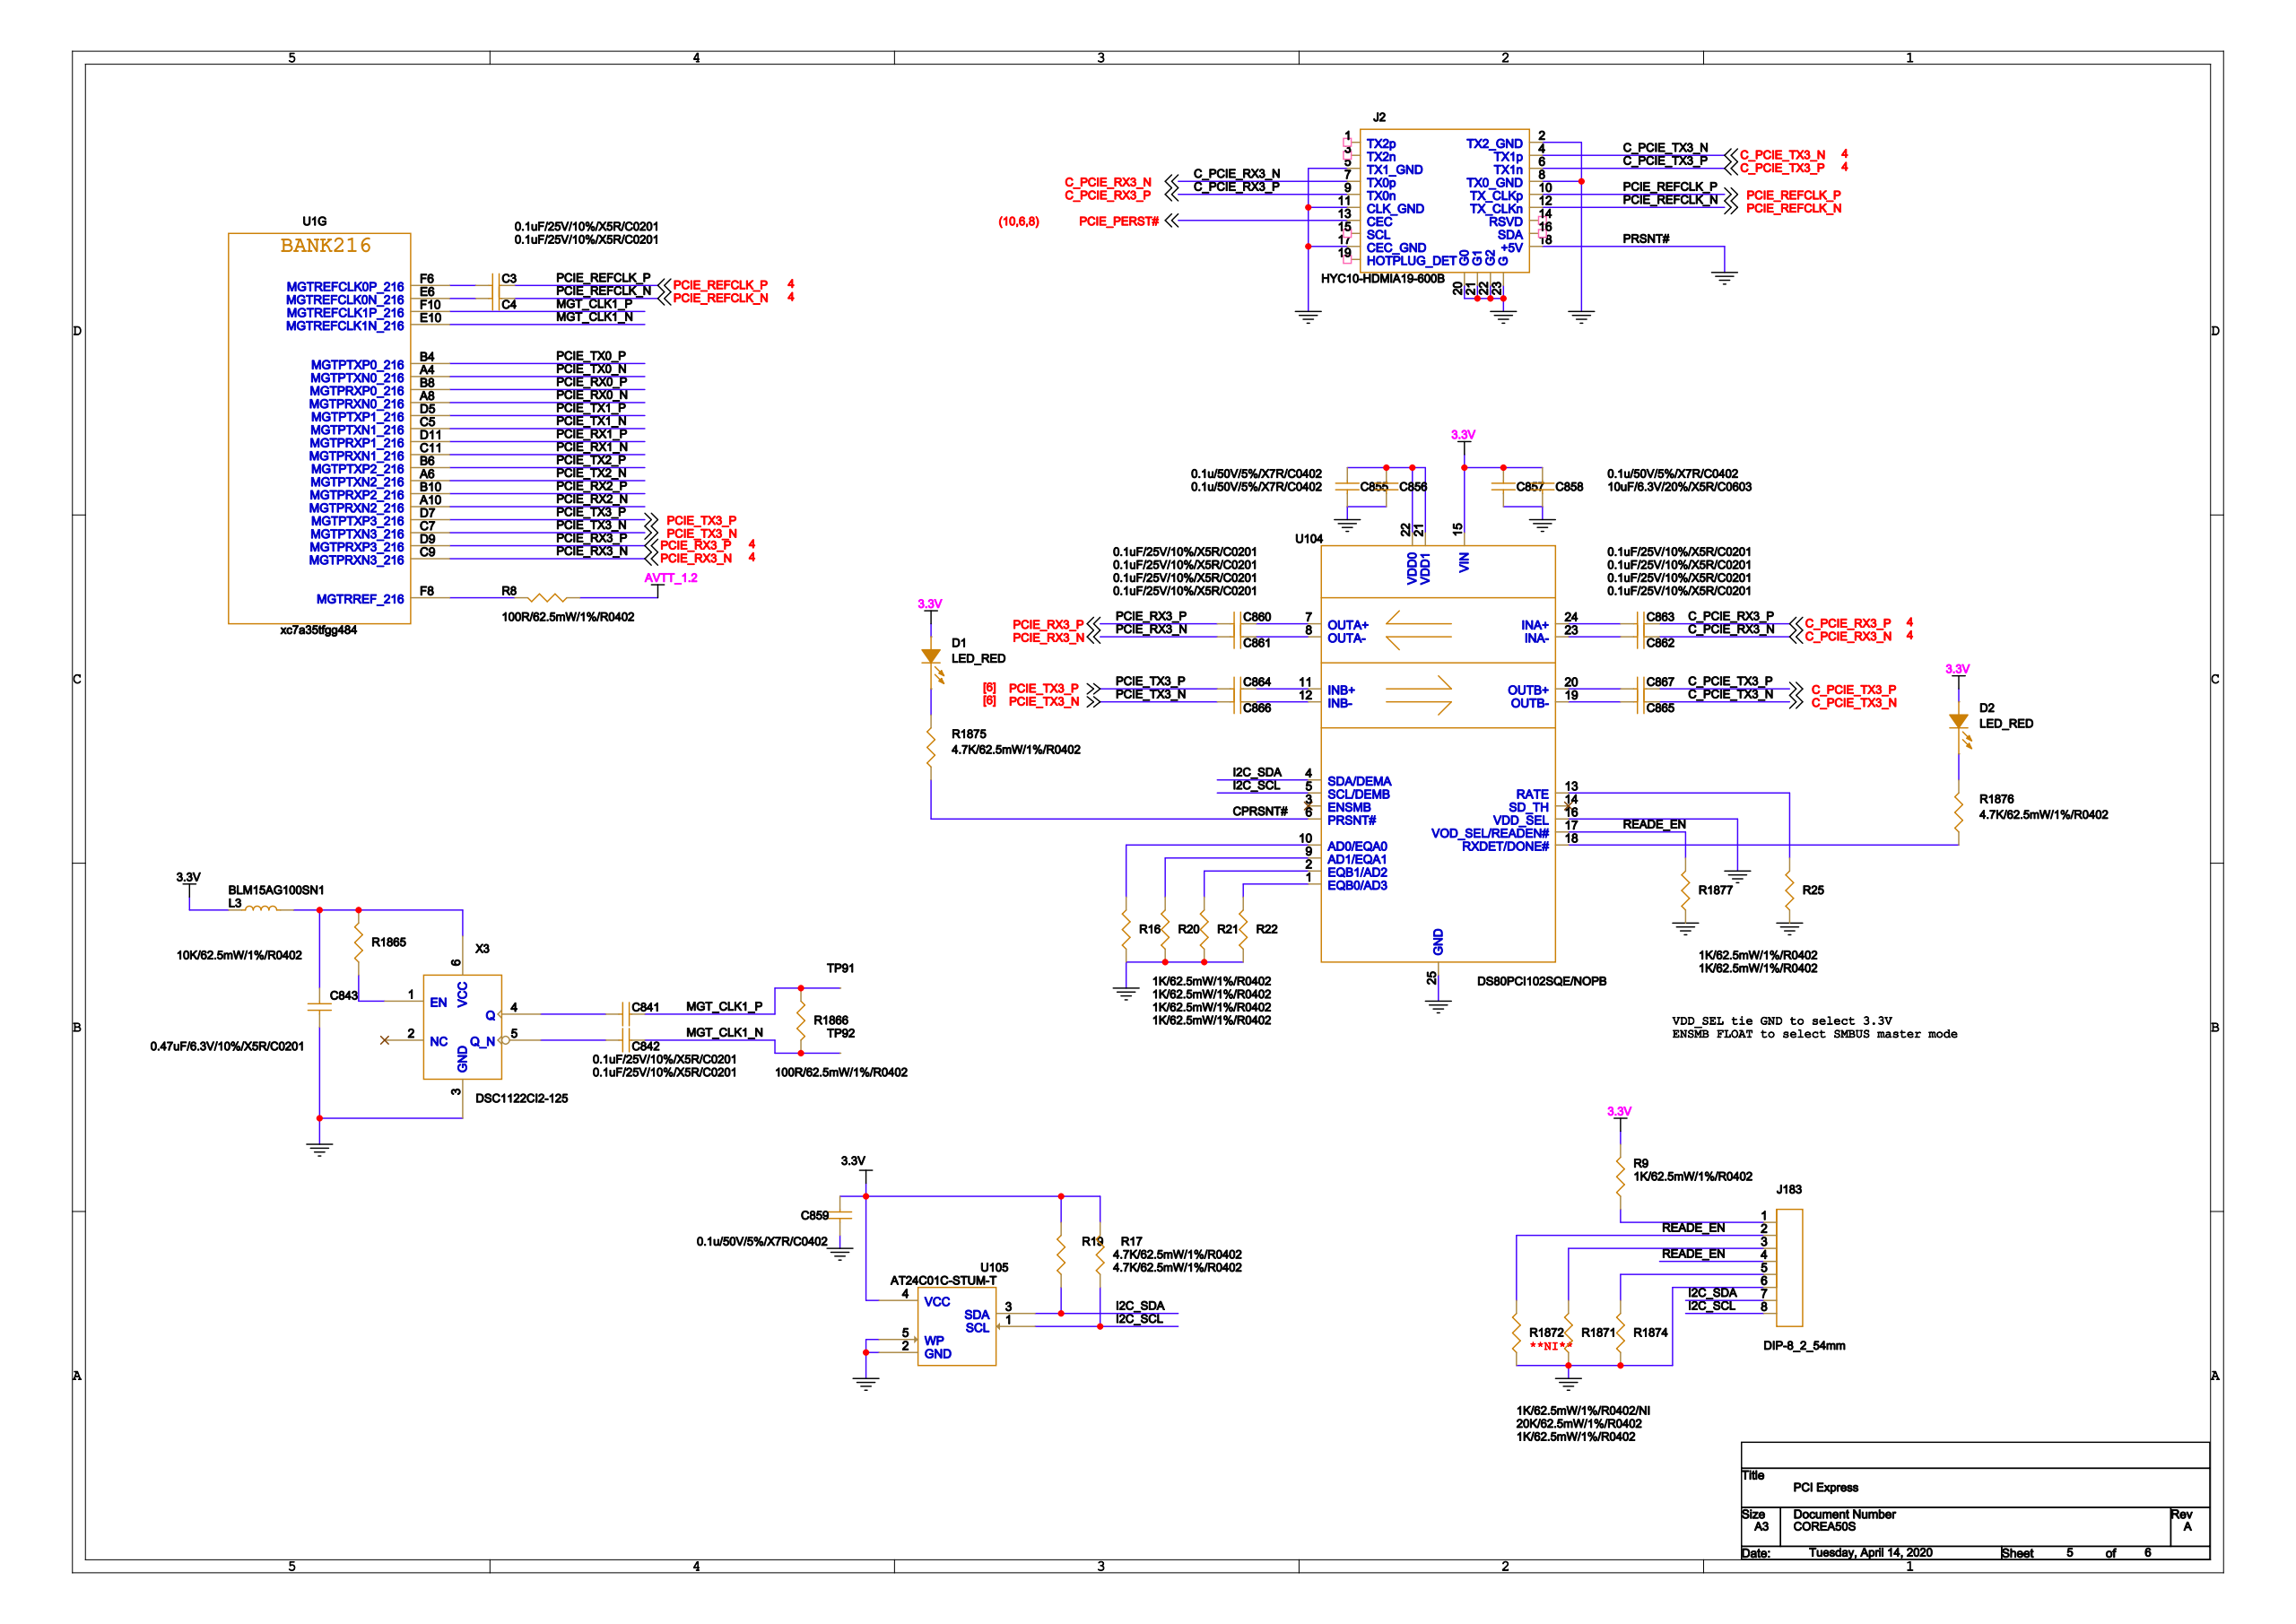Circuit board | Cadence Allegro | 202 parts | 354 nets | one sheet of the schematic
Parts on this sheet (reference | value | footprint):
C3 | 0.1uF/25V/10%/X5R/C0201 | 0201
C4 | 0.1uF/25V/10%/X5R/C0201 | 0201
C841 | 0.1uF/25V/10%/X5R/C0201 | 0201
C842 | 0.1uF/25V/10%/X5R/C0201 | 0201
C843 | 0.47uF/6.3V/10%/X5R/C0201 | 0201
C855 | 0.1u/50V/5%/X7R/C0402 | 0402
C856 | 0.1u/50V/5%/X7R/C0402 | 0402
C857 | 0.1u/50V/5%/X7R/C0402 | 0402
C858 | 10uF/6.3V/20%/X5R/C0603 | 0603
C859 | 0.1u/50V/5%/X7R/C0402 | 0402
C860 | 0.1uF/25V/10%/X5R/C0201 | 0201
C861 | 0.1uF/25V/10%/X5R/C0201 | 0201
C862 | 0.1uF/25V/10%/X5R/C0201 | 0201
C863 | 0.1uF/25V/10%/X5R/C0201 | 0201
C864 | 0.1uF/25V/10%/X5R/C0201 | 0201
C865 | 0.1uF/25V/10%/X5R/C0201 | 0201
C866 | 0.1uF/25V/10%/X5R/C0201 | 0201
C867 | 0.1uF/25V/10%/X5R/C0201 | 0201
D1 | LED_RED | LED0805
D2 | LED_RED | LED0805
J2 | HDMI | HDMI_A1
J183 | DIP-8_2_54mm | DIP8X1
L3 | BLM15AG100SN1 | 0402
R8 | 100R/62.5mW/1%/R0402 | 0402
R9 | 1K/62.5mW/1%/R0402 | 0402
R16 | 1K/62.5mW/1%/R0402 | 0402
R17 | 4.7K/62.5mW/1%/R0402 | 0402
R19 | 4.7K/62.5mW/1%/R0402 | 0402
R20 | 1K/62.5mW/1%/R0402 | 0402
R25 | 1K/62.5mW/1%/R0402 | 0402
R1865 | 10K/62.5mW/1%/R0402 | 0402
R1866 | 100R/62.5mW/1%/R0402 | 0402
R1871 | 20K/62.5mW/1%/R0402 | 0402
R1872 | 1K/62.5mW/1%/R0402 NI** | 0402
R1874 | 1K/62.5mW/1%/R0402 | 0402
R1875 | 4.7K/62.5mW/1%/R0402 | 0402
R1876 | 4.7K/62.5mW/1%/R0402 | 0402
R1877 | 1K/62.5mW/1%/R0402 | 0402
TP91 | TEST POINT A | TEST_12MM
TP92 | TEST POINT A | TEST_12MM
U1 | xc7a35tfgg484 | FGG484_23X23
U104 | DS80PCI102SQE/NOPB | QFN-24_4X4_1
U105 | AT24C01C-STUM-T | SOT_23_5
X3 | DSC1122CI2-125 | VDFN-3225
Nets of these parts (net: part-pin ...):
READE_EN: J183-2 J183-4 R1872-1 R1877-1 U104-17
GND: C843-2 C855-2 C856-2 C857-2 C858-2 C859-2 J2-2 J2-5 J2-8 J2-11 J2-17 J2-18 J2-20 J2-21 J2-22 J2-23 J183-6 R16-2 R20-2 R25-2 R1871-2 R1872-2 R1874-2 R1877-2 U105-2 U105-5 X3-3 U1-A3 U1-C3 U1-R8 U1-R20 U104-16 U104-25
3.3V: C857-1 C858-1 C859-1 D1-1 D2-1 L3-1 R9-1 R17-1 R19-1 U105-4 U104-15
N26580055: D1-2 R1875-1
CPRSNT#: R1875-2 U104-6
I2C_SCL: J183-8 R17-2 U105-1 U104-5
N26580111: D2-2 R1876-1
N26580149: R1876-2 U104-18
I2C_SDA: J183-7 R19-2 U105-3 U104-4
N26574753: J183-3 R1871-1
N26580145: R16-1 U104-10
N26580151: R20-1 U104-9
N26580004: C863-2 U104-24
N26580030: C862-2 U104-23
N26580068: C864-1 U104-11
N26580088: C866-1 U104-12
N26580002: C860-1 U104-7
N26580028: C861-1 U104-8
N26580070: C867-2 U104-20
N26580090: C865-2 U104-19
N26580121: R25-1 U104-13
N26579878: C855-1 C856-1 U104-21 U104-22
N26574769: J183-1 R9-2
N26574520: J183-5 R1874-1
PCIE_PERST#: J2-13
C_PCIE_RX3_P: C863-1 J2-9
C_PCIE_RX3_N: C862-1 J2-7
C_PCIE_TX3_P: C867-1 J2-6
C_PCIE_TX3_N: C865-1 J2-4
PCIE_REFCLK_N: C4-1 J2-12
PCIE_REFCLK_P: C3-1 J2-10
PCIE_RX0_N: U1-A8
PCIE_RX1_N: U1-C11
PCIE_RX2_N: U1-A10
PCIE_RX3_N: C861-2 U1-C9
PCIE_RX0_P: U1-B8
PCIE_RX1_P: U1-D11
PCIE_RX2_P: U1-B10
PCIE_RX3_P: C860-2 U1-D9
PCIE_TX0_N: U1-A4
PCIE_TX1_N: U1-C5
PCIE_TX2_N: U1-A6
PCIE_TX3_N: C866-2 U1-C7
PCIE_TX0_P: U1-B4
PCIE_TX1_P: U1-D5
PCIE_TX2_P: U1-B6
PCIE_TX3_P: C864-2 U1-D7
N26369927: C4-2 U1-E6
N26369910: C3-2 U1-F6
MGT_CLK1_N: C842-1 R1866-1 TP92-1 U1-E10
MGT_CLK1_P: C841-1 R1866-2 TP91-1 U1-F10
N26370273: R8-2 U1-F8
AVTT_1.2: R8-1 U1-C4
N26530968: R1865-1 X3-1
N26530950: C843-1 L3-2 R1865-2 X3-6
N26531005: C841-2 X3-4
N26531024: C842-2 X3-5